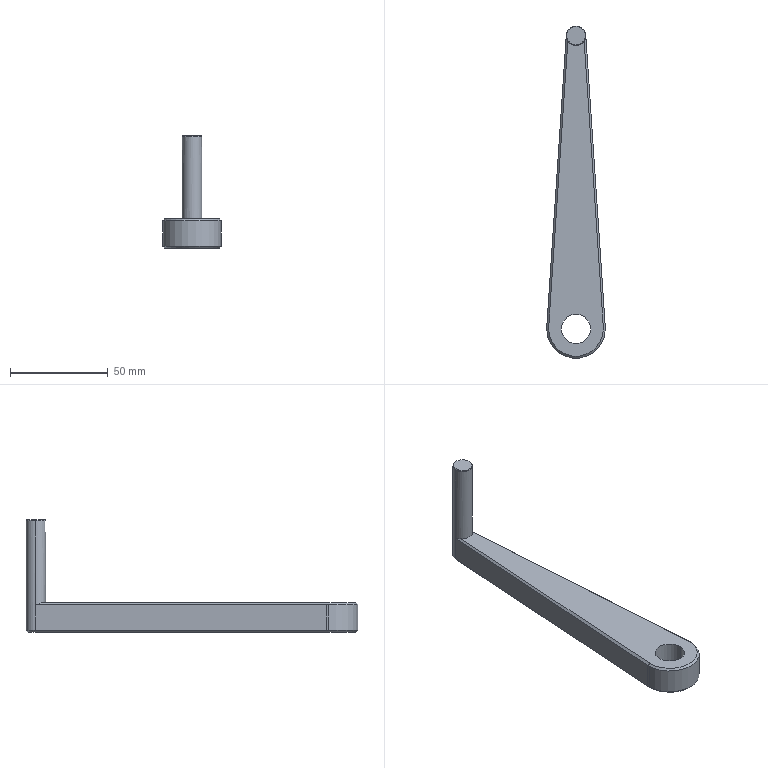Part | SolidWorks | features BaseBody 1 | 1 solid | 27 faces | box 30 x 170 x 57.5 mm | volume 51323 mm3 | cone 11 | plane 9 | cylinder 7 | commonest cylinder face diameters 30 x3 10 x2 15 x2
STEP:
#1=CARTESIAN_POINT('',(-4.823,150.,57.427));
#2=VERTEX_POINT('',#1);
#3=CARTESIAN_POINT('',(4.823,150.,57.427));
#4=VERTEX_POINT('',#3);
#5=CARTESIAN_POINT('',(0.,150.,57.427));
#6=DIRECTION('',(0.,0.,-1.));
#7=DIRECTION('',(-1.,0.,0.));
#8=AXIS2_PLACEMENT_3D('',#5,#6,#7);
#9=CIRCLE('',#8,4.823);
#10=EDGE_CURVE('',#2,#4,#9,.T.);
#11=ORIENTED_EDGE('',*,*,#10,.T.);
#12=CARTESIAN_POINT('',(5.,150.,57.));
#13=VERTEX_POINT('',#12);
#14=CARTESIAN_POINT('',(4.912,150.,57.213));
#15=DIRECTION('',(0.3827,0.,-0.9239));
#16=VECTOR('',#15,1000.);
#17=LINE('',#14,#16);
#18=EDGE_CURVE('',#4,#13,#17,.T.);
#19=ORIENTED_EDGE('',*,*,#18,.T.);
#20=CARTESIAN_POINT('',(-5.,150.,57.));
#21=VERTEX_POINT('',#20);
#22=CARTESIAN_POINT('',(0.,150.,57.));
#23=DIRECTION('',(0.,0.,1.));
#24=DIRECTION('',(-1.,0.,0.));
#25=AXIS2_PLACEMENT_3D('',#22,#23,#24);
#26=CIRCLE('',#25,5.);
#27=EDGE_CURVE('',#13,#21,#26,.T.);
#28=ORIENTED_EDGE('',*,*,#27,.T.);
#29=CARTESIAN_POINT('',(-4.912,150.,57.213));
#30=DIRECTION('',(-0.3827,0.,-0.9239));
#31=VECTOR('',#30,1000.);
#32=LINE('',#29,#31);
#33=EDGE_CURVE('',#2,#21,#32,.T.);
#34=ORIENTED_EDGE('',*,*,#33,.F.);
#35=EDGE_LOOP('',(#11,#19,#28,#34));
#36=FACE_OUTER_BOUND('',#35,.T.);
#37=CARTESIAN_POINT('',(0.,150.,57.213));
#38=DIRECTION('',(0.,0.,-1.));
#39=DIRECTION('',(-1.,0.,0.));
#40=AXIS2_PLACEMENT_3D('',#37,#38,#39);
#41=CONICAL_SURFACE('',#40,4.912,0.3927);
#42=ADVANCED_FACE('',(#36),#41,.T.);
#43=CARTESIAN_POINT('',(-4.75,150.,57.5));
#44=VERTEX_POINT('',#43);
#45=CARTESIAN_POINT('',(4.75,150.,57.5));
#46=VERTEX_POINT('',#45);
#47=CARTESIAN_POINT('',(0.,150.,57.5));
#48=DIRECTION('',(0.,0.,-1.));
#49=DIRECTION('',(-1.,0.,0.));
#50=AXIS2_PLACEMENT_3D('',#47,#48,#49);
#51=CIRCLE('',#50,4.75);
#52=EDGE_CURVE('',#44,#46,#51,.T.);
#53=ORIENTED_EDGE('',*,*,#52,.T.);
#54=CARTESIAN_POINT('',(4.875,150.,57.375));
#55=DIRECTION('',(0.7071,0.,-0.7071));
#56=VECTOR('',#55,1000.);
#57=LINE('',#54,#56);
#58=EDGE_CURVE('',#46,#4,#57,.T.);
#59=ORIENTED_EDGE('',*,*,#58,.T.);
#60=ORIENTED_EDGE('',*,*,#10,.F.);
#61=CARTESIAN_POINT('',(-4.875,150.,57.375));
#62=DIRECTION('',(-0.7071,0.,-0.7071));
#63=VECTOR('',#62,1000.);
#64=LINE('',#61,#63);
#65=EDGE_CURVE('',#44,#2,#64,.T.);
#66=ORIENTED_EDGE('',*,*,#65,.F.);
#67=EDGE_LOOP('',(#53,#59,#60,#66));
#68=FACE_OUTER_BOUND('',#67,.T.);
#69=CARTESIAN_POINT('',(0.,150.,57.375));
#70=DIRECTION('',(0.,0.,-1.));
#71=DIRECTION('',(-1.,0.,0.));
#72=AXIS2_PLACEMENT_3D('',#69,#70,#71);
#73=CONICAL_SURFACE('',#72,4.875,0.7854);
#74=ADVANCED_FACE('',(#68),#73,.T.);
#75=CARTESIAN_POINT('',(0.,150.,57.));
#76=DIRECTION('',(0.,0.,1.));
#77=DIRECTION('',(-1.,0.,0.));
#78=AXIS2_PLACEMENT_3D('',#75,#76,#77);
#79=CIRCLE('',#78,5.);
#80=EDGE_CURVE('',#21,#13,#79,.T.);
#81=ORIENTED_EDGE('',*,*,#80,.F.);
#82=CARTESIAN_POINT('',(-5.,150.,14.011));
#83=VERTEX_POINT('',#82);
#84=CARTESIAN_POINT('',(-5.,150.,0.));
#85=DIRECTION('',(0.,0.,-1.));
#86=VECTOR('',#85,1000.);
#87=LINE('',#84,#86);
#88=EDGE_CURVE('',#21,#83,#87,.T.);
#89=ORIENTED_EDGE('',*,*,#88,.T.);
#90=CARTESIAN_POINT('',(-4.191,147.273,15.));
#91=VERTEX_POINT('',#90);
#92=CARTESIAN_POINT('',(-4.191,147.273,15.));
#93=CARTESIAN_POINT('',(-4.723,148.091,14.415));
#94=CARTESIAN_POINT('',(-5.,149.025,14.076));
#95=CARTESIAN_POINT('',(-5.,150.,14.011));
#96=(BOUNDED_CURVE()B_SPLINE_CURVE(3,(#92,#93,#94,#95),.UNSPECIFIED.,.F.,.T.)B_SPLINE_CURVE_WITH_KNOTS((4,4),(2.498,3.075),.UNSPECIFIED.)CURVE()GEOMETRIC_REPRESENTATION_ITEM()RATIONAL_B_SPLINE_CURVE((1.,0.9725,0.9725,1.))REPRESENTATION_ITEM(''));
#97=EDGE_CURVE('',#91,#83,#96,.T.);
#98=ORIENTED_EDGE('',*,*,#97,.F.);
#99=CARTESIAN_POINT('',(4.191,147.273,15.));
#100=VERTEX_POINT('',#99);
#101=CARTESIAN_POINT('',(0.,150.,15.));
#102=DIRECTION('',(0.,0.,-1.));
#103=DIRECTION('',(-1.,0.,0.));
#104=AXIS2_PLACEMENT_3D('',#101,#102,#103);
#105=CIRCLE('',#104,5.);
#106=EDGE_CURVE('',#100,#91,#105,.T.);
#107=ORIENTED_EDGE('',*,*,#106,.F.);
#108=CARTESIAN_POINT('',(5.,150.,14.011));
#109=VERTEX_POINT('',#108);
#110=CARTESIAN_POINT('',(5.,150.,14.011));
#111=CARTESIAN_POINT('',(5.,149.025,14.076));
#112=CARTESIAN_POINT('',(4.723,148.091,14.415));
#113=CARTESIAN_POINT('',(4.191,147.273,15.));
#114=(BOUNDED_CURVE()B_SPLINE_CURVE(3,(#110,#111,#112,#113),.UNSPECIFIED.,.F.,.F.)B_SPLINE_CURVE_WITH_KNOTS((4,4),(0.06672,0.6435),.UNSPECIFIED.)CURVE()GEOMETRIC_REPRESENTATION_ITEM()RATIONAL_B_SPLINE_CURVE((1.,0.9725,0.9725,1.))REPRESENTATION_ITEM(''));
#115=EDGE_CURVE('',#109,#100,#114,.T.);
#116=ORIENTED_EDGE('',*,*,#115,.F.);
#117=CARTESIAN_POINT('',(5.,150.,0.));
#118=DIRECTION('',(0.,0.,-1.));
#119=VECTOR('',#118,1000.);
#120=LINE('',#117,#119);
#121=EDGE_CURVE('',#13,#109,#120,.T.);
#122=ORIENTED_EDGE('',*,*,#121,.F.);
#123=EDGE_LOOP('',(#81,#89,#98,#107,#116,#122));
#124=FACE_OUTER_BOUND('',#123,.T.);
#125=CARTESIAN_POINT('',(0.,150.,0.));
#126=DIRECTION('',(0.,0.,-1.));
#127=DIRECTION('',(1.,0.,0.));
#128=AXIS2_PLACEMENT_3D('',#125,#126,#127);
#129=CYLINDRICAL_SURFACE('',#128,5.);
#130=ADVANCED_FACE('',(#124),#129,.T.);
#131=CARTESIAN_POINT('',(-13.969,0.9333,0.));
#132=VERTEX_POINT('',#131);
#133=CARTESIAN_POINT('',(-14.,0.,0.));
#134=VERTEX_POINT('',#133);
#135=CARTESIAN_POINT('',(0.,0.,0.));
#136=DIRECTION('',(0.,0.,1.));
#137=DIRECTION('',(1.,0.,0.));
#138=AXIS2_PLACEMENT_3D('',#135,#136,#137);
#139=CIRCLE('',#138,14.);
#140=EDGE_CURVE('',#132,#134,#139,.T.);
#141=ORIENTED_EDGE('',*,*,#140,.T.);
#142=CARTESIAN_POINT('',(-15.,0.,1.));
#143=VERTEX_POINT('',#142);
#144=CARTESIAN_POINT('',(-14.5,0.,0.5));
#145=DIRECTION('',(-0.7071,0.,0.7071));
#146=VECTOR('',#145,1000.);
#147=LINE('',#144,#146);
#148=EDGE_CURVE('',#134,#143,#147,.T.);
#149=ORIENTED_EDGE('',*,*,#148,.T.);
#150=CARTESIAN_POINT('',(-14.967,1.,1.));
#151=VERTEX_POINT('',#150);
#152=CARTESIAN_POINT('',(0.,0.,1.));
#153=DIRECTION('',(0.,0.,-1.));
#154=DIRECTION('',(1.,0.,0.));
#155=AXIS2_PLACEMENT_3D('',#152,#153,#154);
#156=CIRCLE('',#155,15.);
#157=EDGE_CURVE('',#143,#151,#156,.T.);
#158=ORIENTED_EDGE('',*,*,#157,.T.);
#159=CARTESIAN_POINT('',(-13.969,0.9333,0.));
#160=DIRECTION('',(-0.7055,0.04714,0.7071));
#161=VECTOR('',#160,1000.);
#162=LINE('',#159,#161);
#163=EDGE_CURVE('',#132,#151,#162,.T.);
#164=ORIENTED_EDGE('',*,*,#163,.F.);
#165=EDGE_LOOP('',(#141,#149,#158,#164));
#166=FACE_OUTER_BOUND('',#165,.T.);
#167=CARTESIAN_POINT('',(0.,0.,0.5));
#168=DIRECTION('',(0.,0.,1.));
#169=DIRECTION('',(1.,0.,0.));
#170=AXIS2_PLACEMENT_3D('',#167,#168,#169);
#171=CONICAL_SURFACE('',#170,14.5,0.7854);
#172=ADVANCED_FACE('',(#166),#171,.T.);
#173=ORIENTED_EDGE('',*,*,#148,.F.);
#174=CARTESIAN_POINT('',(14.,0.,0.));
#175=VERTEX_POINT('',#174);
#176=CARTESIAN_POINT('',(0.,0.,0.));
#177=DIRECTION('',(0.,0.,1.));
#178=DIRECTION('',(1.,0.,0.));
#179=AXIS2_PLACEMENT_3D('',#176,#177,#178);
#180=CIRCLE('',#179,14.);
#181=EDGE_CURVE('',#134,#175,#180,.T.);
#182=ORIENTED_EDGE('',*,*,#181,.T.);
#183=CARTESIAN_POINT('',(15.,0.,1.));
#184=VERTEX_POINT('',#183);
#185=CARTESIAN_POINT('',(14.5,0.,0.5));
#186=DIRECTION('',(0.7071,0.,0.7071));
#187=VECTOR('',#186,1000.);
#188=LINE('',#185,#187);
#189=EDGE_CURVE('',#175,#184,#188,.T.);
#190=ORIENTED_EDGE('',*,*,#189,.T.);
#191=CARTESIAN_POINT('',(0.,0.,1.));
#192=DIRECTION('',(0.,0.,-1.));
#193=DIRECTION('',(1.,0.,0.));
#194=AXIS2_PLACEMENT_3D('',#191,#192,#193);
#195=CIRCLE('',#194,15.);
#196=EDGE_CURVE('',#184,#143,#195,.T.);
#197=ORIENTED_EDGE('',*,*,#196,.T.);
#198=EDGE_LOOP('',(#173,#182,#190,#197));
#199=FACE_OUTER_BOUND('',#198,.T.);
#200=CARTESIAN_POINT('',(0.,0.,0.5));
#201=DIRECTION('',(0.,0.,1.));
#202=DIRECTION('',(1.,0.,0.));
#203=AXIS2_PLACEMENT_3D('',#200,#201,#202);
#204=CONICAL_SURFACE('',#203,14.5,0.7854);
#205=ADVANCED_FACE('',(#199),#204,.T.);
#206=CARTESIAN_POINT('',(-15.,0.,14.));
#207=VERTEX_POINT('',#206);
#208=CARTESIAN_POINT('',(15.,0.,14.));
#209=VERTEX_POINT('',#208);
#210=CARTESIAN_POINT('',(0.,0.,14.));
#211=DIRECTION('',(0.,0.,1.));
#212=DIRECTION('',(1.,0.,0.));
#213=AXIS2_PLACEMENT_3D('',#210,#211,#212);
#214=CIRCLE('',#213,15.);
#215=EDGE_CURVE('',#207,#209,#214,.T.);
#216=ORIENTED_EDGE('',*,*,#215,.F.);
#217=CARTESIAN_POINT('',(-15.,0.,0.));
#218=DIRECTION('',(0.,0.,-1.));
#219=VECTOR('',#218,1000.);
#220=LINE('',#217,#219);
#221=EDGE_CURVE('',#207,#143,#220,.T.);
#222=ORIENTED_EDGE('',*,*,#221,.T.);
#223=ORIENTED_EDGE('',*,*,#196,.F.);
#224=CARTESIAN_POINT('',(15.,0.,0.));
#225=DIRECTION('',(0.,0.,-1.));
#226=VECTOR('',#225,1000.);
#227=LINE('',#224,#226);
#228=EDGE_CURVE('',#209,#184,#227,.T.);
#229=ORIENTED_EDGE('',*,*,#228,.F.);
#230=EDGE_LOOP('',(#216,#222,#223,#229));
#231=FACE_OUTER_BOUND('',#230,.T.);
#232=CARTESIAN_POINT('',(0.,0.,0.));
#233=DIRECTION('',(0.,0.,-1.));
#234=DIRECTION('',(1.,0.,0.));
#235=AXIS2_PLACEMENT_3D('',#232,#233,#234);
#236=CYLINDRICAL_SURFACE('',#235,15.);
#237=ADVANCED_FACE('',(#231),#236,.T.);
#238=CARTESIAN_POINT('',(14.967,1.,14.));
#239=VERTEX_POINT('',#238);
#240=CARTESIAN_POINT('',(0.,0.,14.));
#241=DIRECTION('',(0.,0.,1.));
#242=DIRECTION('',(1.,0.,0.));
#243=AXIS2_PLACEMENT_3D('',#240,#241,#242);
#244=CIRCLE('',#243,15.);
#245=EDGE_CURVE('',#209,#239,#244,.T.);
#246=ORIENTED_EDGE('',*,*,#245,.F.);
#247=ORIENTED_EDGE('',*,*,#228,.T.);
#248=CARTESIAN_POINT('',(14.967,1.,1.));
#249=VERTEX_POINT('',#248);
#250=CARTESIAN_POINT('',(0.,0.,1.));
#251=DIRECTION('',(0.,0.,-1.));
#252=DIRECTION('',(1.,0.,0.));
#253=AXIS2_PLACEMENT_3D('',#250,#251,#252);
#254=CIRCLE('',#253,15.);
#255=EDGE_CURVE('',#249,#184,#254,.T.);
#256=ORIENTED_EDGE('',*,*,#255,.F.);
#257=CARTESIAN_POINT('',(14.967,1.,0.));
#258=DIRECTION('',(0.,0.,1.));
#259=VECTOR('',#258,1000.);
#260=LINE('',#257,#259);
#261=EDGE_CURVE('',#249,#239,#260,.T.);
#262=ORIENTED_EDGE('',*,*,#261,.T.);
#263=EDGE_LOOP('',(#246,#247,#256,#262));
#264=FACE_OUTER_BOUND('',#263,.T.);
#265=CARTESIAN_POINT('',(0.,0.,0.));
#266=DIRECTION('',(0.,0.,-1.));
#267=DIRECTION('',(1.,0.,0.));
#268=AXIS2_PLACEMENT_3D('',#265,#266,#267);
#269=CYLINDRICAL_SURFACE('',#268,15.);
#270=ADVANCED_FACE('',(#264),#269,.T.);
#271=CARTESIAN_POINT('',(14.,0.,15.));
#272=VERTEX_POINT('',#271);
#273=CARTESIAN_POINT('',(-14.,0.,15.));
#274=VERTEX_POINT('',#273);
#275=CARTESIAN_POINT('',(0.,0.,15.));
#276=DIRECTION('',(0.,0.,-1.));
#277=DIRECTION('',(1.,0.,0.));
#278=AXIS2_PLACEMENT_3D('',#275,#276,#277);
#279=CIRCLE('',#278,14.);
#280=EDGE_CURVE('',#272,#274,#279,.T.);
#281=ORIENTED_EDGE('',*,*,#280,.T.);
#282=CARTESIAN_POINT('',(-14.5,0.,14.5));
#283=DIRECTION('',(-0.7071,0.,-0.7071));
#284=VECTOR('',#283,1000.);
#285=LINE('',#282,#284);
#286=EDGE_CURVE('',#274,#207,#285,.T.);
#287=ORIENTED_EDGE('',*,*,#286,.T.);
#288=ORIENTED_EDGE('',*,*,#215,.T.);
#289=CARTESIAN_POINT('',(14.5,0.,14.5));
#290=DIRECTION('',(0.7071,0.,-0.7071));
#291=VECTOR('',#290,1000.);
#292=LINE('',#289,#291);
#293=EDGE_CURVE('',#272,#209,#292,.T.);
#294=ORIENTED_EDGE('',*,*,#293,.F.);
#295=EDGE_LOOP('',(#281,#287,#288,#294));
#296=FACE_OUTER_BOUND('',#295,.T.);
#297=CARTESIAN_POINT('',(0.,0.,14.5));
#298=DIRECTION('',(0.,0.,-1.));
#299=DIRECTION('',(1.,0.,0.));
#300=AXIS2_PLACEMENT_3D('',#297,#298,#299);
#301=CONICAL_SURFACE('',#300,14.5,0.7854);
#302=ADVANCED_FACE('',(#296),#301,.T.);
#303=CARTESIAN_POINT('',(13.969,0.9333,15.));
#304=VERTEX_POINT('',#303);
#305=CARTESIAN_POINT('',(0.,0.,15.));
#306=DIRECTION('',(0.,0.,-1.));
#307=DIRECTION('',(1.,0.,0.));
#308=AXIS2_PLACEMENT_3D('',#305,#306,#307);
#309=CIRCLE('',#308,14.);
#310=EDGE_CURVE('',#304,#272,#309,.T.);
#311=ORIENTED_EDGE('',*,*,#310,.T.);
#312=ORIENTED_EDGE('',*,*,#293,.T.);
#313=ORIENTED_EDGE('',*,*,#245,.T.);
#314=CARTESIAN_POINT('',(14.967,1.,14.));
#315=DIRECTION('',(-0.7055,-0.04714,0.7071));
#316=VECTOR('',#315,1000.);
#317=LINE('',#314,#316);
#318=EDGE_CURVE('',#239,#304,#317,.T.);
#319=ORIENTED_EDGE('',*,*,#318,.T.);
#320=EDGE_LOOP('',(#311,#312,#313,#319));
#321=FACE_OUTER_BOUND('',#320,.T.);
#322=CARTESIAN_POINT('',(0.,0.,14.5));
#323=DIRECTION('',(0.,0.,-1.));
#324=DIRECTION('',(1.,0.,0.));
#325=AXIS2_PLACEMENT_3D('',#322,#323,#324);
#326=CONICAL_SURFACE('',#325,14.5,0.7854);
#327=ADVANCED_FACE('',(#321),#326,.T.);
#328=CARTESIAN_POINT('',(7.5,0.,0.));
#329=VERTEX_POINT('',#328);
#330=CARTESIAN_POINT('',(-7.5,0.,0.));
#331=VERTEX_POINT('',#330);
#332=CARTESIAN_POINT('',(0.,0.,0.));
#333=DIRECTION('',(0.,0.,1.));
#334=DIRECTION('',(-1.,0.,0.));
#335=AXIS2_PLACEMENT_3D('',#332,#333,#334);
#336=CIRCLE('',#335,7.5);
#337=EDGE_CURVE('',#329,#331,#336,.T.);
#338=ORIENTED_EDGE('',*,*,#337,.F.);
#339=CARTESIAN_POINT('',(7.5,0.,15.));
#340=VERTEX_POINT('',#339);
#341=CARTESIAN_POINT('',(7.5,0.,15.));
#342=DIRECTION('',(0.,0.,1.));
#343=VECTOR('',#342,1000.);
#344=LINE('',#341,#343);
#345=EDGE_CURVE('',#329,#340,#344,.T.);
#346=ORIENTED_EDGE('',*,*,#345,.T.);
#347=CARTESIAN_POINT('',(-7.5,0.,15.));
#348=VERTEX_POINT('',#347);
#349=CARTESIAN_POINT('',(0.,0.,15.));
#350=DIRECTION('',(0.,0.,-1.));
#351=DIRECTION('',(-1.,0.,0.));
#352=AXIS2_PLACEMENT_3D('',#349,#350,#351);
#353=CIRCLE('',#352,7.5);
#354=EDGE_CURVE('',#348,#340,#353,.T.);
#355=ORIENTED_EDGE('',*,*,#354,.F.);
#356=CARTESIAN_POINT('',(-7.5,0.,15.));
#357=DIRECTION('',(0.,0.,1.));
#358=VECTOR('',#357,1000.);
#359=LINE('',#356,#358);
#360=EDGE_CURVE('',#331,#348,#359,.T.);
#361=ORIENTED_EDGE('',*,*,#360,.F.);
#362=EDGE_LOOP('',(#338,#346,#355,#361));
#363=FACE_OUTER_BOUND('',#362,.T.);
#364=CARTESIAN_POINT('',(0.,0.,15.));
#365=DIRECTION('',(0.,0.,1.));
#366=DIRECTION('',(-1.,0.,0.));
#367=AXIS2_PLACEMENT_3D('',#364,#365,#366);
#368=CYLINDRICAL_SURFACE('',#367,7.5);
#369=ADVANCED_FACE('',(#363),#368,.F.);
#370=CARTESIAN_POINT('',(3.991,150.267,0.));
#371=VERTEX_POINT('',#370);
#372=CARTESIAN_POINT('',(4.989,150.333,1.));
#373=VERTEX_POINT('',#372);
#374=CARTESIAN_POINT('',(3.991,150.267,0.));
#375=DIRECTION('',(0.7055,0.04714,0.7071));
#376=VECTOR('',#375,1000.);
#377=LINE('',#374,#376);
#378=EDGE_CURVE('',#371,#373,#377,.T.);
#379=ORIENTED_EDGE('',*,*,#378,.T.);
#380=CARTESIAN_POINT('',(9.978,75.667,1.));
#381=DIRECTION('',(0.06667,-0.9978,0.));
#382=VECTOR('',#381,1000.);
#383=LINE('',#380,#382);
#384=EDGE_CURVE('',#373,#249,#383,.T.);
#385=ORIENTED_EDGE('',*,*,#384,.T.);
#386=CARTESIAN_POINT('',(13.969,0.9333,0.));
#387=VERTEX_POINT('',#386);
#388=CARTESIAN_POINT('',(14.967,1.,1.));
#389=DIRECTION('',(-0.7055,-0.04714,-0.7071));
#390=VECTOR('',#389,1000.);
#391=LINE('',#388,#390);
#392=EDGE_CURVE('',#249,#387,#391,.T.);
#393=ORIENTED_EDGE('',*,*,#392,.T.);
#394=CARTESIAN_POINT('',(8.98,75.6,0.));
#395=DIRECTION('',(-0.06667,0.9978,0.));
#396=VECTOR('',#395,1000.);
#397=LINE('',#394,#396);
#398=EDGE_CURVE('',#387,#371,#397,.T.);
#399=ORIENTED_EDGE('',*,*,#398,.T.);
#400=EDGE_LOOP('',(#379,#385,#393,#399));
#401=FACE_OUTER_BOUND('',#400,.T.);
#402=CARTESIAN_POINT('',(9.479,75.633,0.5));
#403=DIRECTION('',(0.7055,0.04714,-0.7071));
#404=DIRECTION('',(0.,-0.9978,-0.06652));
#405=AXIS2_PLACEMENT_3D('',#402,#403,#404);
#406=PLANE('',#405);
#407=ADVANCED_FACE('',(#401),#406,.T.);
#408=CARTESIAN_POINT('',(-3.991,150.267,0.));
#409=VERTEX_POINT('',#408);
#410=CARTESIAN_POINT('',(-4.989,150.333,1.));
#411=VERTEX_POINT('',#410);
#412=CARTESIAN_POINT('',(-3.991,150.267,0.));
#413=DIRECTION('',(-0.7055,0.04714,0.7071));
#414=VECTOR('',#413,1000.);
#415=LINE('',#412,#414);
#416=EDGE_CURVE('',#409,#411,#415,.T.);
#417=ORIENTED_EDGE('',*,*,#416,.T.);
#418=CARTESIAN_POINT('',(0.,150.,1.));
#419=DIRECTION('',(0.,0.,-1.));
#420=DIRECTION('',(1.,0.,0.));
#421=AXIS2_PLACEMENT_3D('',#418,#419,#420);
#422=CIRCLE('',#421,5.);
#423=EDGE_CURVE('',#411,#373,#422,.T.);
#424=ORIENTED_EDGE('',*,*,#423,.T.);
#425=ORIENTED_EDGE('',*,*,#378,.F.);
#426=CARTESIAN_POINT('',(0.,150.,0.));
#427=DIRECTION('',(0.,0.,1.));
#428=DIRECTION('',(1.,0.,0.));
#429=AXIS2_PLACEMENT_3D('',#426,#427,#428);
#430=CIRCLE('',#429,4.);
#431=EDGE_CURVE('',#371,#409,#430,.T.);
#432=ORIENTED_EDGE('',*,*,#431,.T.);
#433=EDGE_LOOP('',(#417,#424,#425,#432));
#434=FACE_OUTER_BOUND('',#433,.T.);
#435=CARTESIAN_POINT('',(0.,150.,0.5));
#436=DIRECTION('',(0.,0.,1.));
#437=DIRECTION('',(1.,0.,0.));
#438=AXIS2_PLACEMENT_3D('',#435,#436,#437);
#439=CONICAL_SURFACE('',#438,4.5,0.7854);
#440=ADVANCED_FACE('',(#434),#439,.T.);
#441=ORIENTED_EDGE('',*,*,#163,.T.);
#442=CARTESIAN_POINT('',(-4.989,150.333,1.));
#443=DIRECTION('',(0.06667,0.9978,0.));
#444=VECTOR('',#443,1000.);
#445=LINE('',#442,#444);
#446=EDGE_CURVE('',#151,#411,#445,.T.);
#447=ORIENTED_EDGE('',*,*,#446,.T.);
#448=ORIENTED_EDGE('',*,*,#416,.F.);
#449=CARTESIAN_POINT('',(-3.991,150.267,0.));
#450=DIRECTION('',(-0.06667,-0.9978,0.));
#451=VECTOR('',#450,1000.);
#452=LINE('',#449,#451);
#453=EDGE_CURVE('',#409,#132,#452,.T.);
#454=ORIENTED_EDGE('',*,*,#453,.T.);
#455=EDGE_LOOP('',(#441,#447,#448,#454));
#456=FACE_OUTER_BOUND('',#455,.T.);
#457=CARTESIAN_POINT('',(-4.49,150.3,0.5));
#458=DIRECTION('',(-0.7055,0.04714,-0.7071));
#459=DIRECTION('',(-0.7079,0.,0.7063));
#460=AXIS2_PLACEMENT_3D('',#457,#458,#459);
#461=PLANE('',#460);
#462=ADVANCED_FACE('',(#456),#461,.T.);
#463=ORIENTED_EDGE('',*,*,#384,.F.);
#464=CARTESIAN_POINT('',(4.989,150.333,14.));
#465=VERTEX_POINT('',#464);
#466=CARTESIAN_POINT('',(4.989,150.333,0.));
#467=DIRECTION('',(0.,0.,1.));
#468=VECTOR('',#467,1000.);
#469=LINE('',#466,#468);
#470=EDGE_CURVE('',#373,#465,#469,.T.);
#471=ORIENTED_EDGE('',*,*,#470,.T.);
#472=CARTESIAN_POINT('',(9.978,75.667,14.));
#473=DIRECTION('',(-0.06667,0.9978,0.));
#474=VECTOR('',#473,1000.);
#475=LINE('',#472,#474);
#476=EDGE_CURVE('',#239,#465,#475,.T.);
#477=ORIENTED_EDGE('',*,*,#476,.F.);
#478=ORIENTED_EDGE('',*,*,#261,.F.);
#479=EDGE_LOOP('',(#463,#471,#477,#478));
#480=FACE_OUTER_BOUND('',#479,.T.);
#481=CARTESIAN_POINT('',(14.967,1.,0.));
#482=DIRECTION('',(0.9978,0.06667,0.));
#483=DIRECTION('',(0.,0.,-1.));
#484=AXIS2_PLACEMENT_3D('',#481,#482,#483);
#485=PLANE('',#484);
#486=ADVANCED_FACE('',(#480),#485,.T.);
#487=CARTESIAN_POINT('',(0.,0.,0.));
#488=DIRECTION('',(0.,0.,1.));
#489=DIRECTION('',(-1.,0.,0.));
#490=AXIS2_PLACEMENT_3D('',#487,#488,#489);
#491=CIRCLE('',#490,7.5);
#492=EDGE_CURVE('',#331,#329,#491,.T.);
#493=ORIENTED_EDGE('',*,*,#492,.T.);
#494=ORIENTED_EDGE('',*,*,#337,.T.);
#495=EDGE_LOOP('',(#493,#494));
#496=FACE_BOUND('',#495,.T.);
#497=ORIENTED_EDGE('',*,*,#398,.F.);
#498=CARTESIAN_POINT('',(0.,0.,0.));
#499=DIRECTION('',(0.,0.,1.));
#500=DIRECTION('',(1.,0.,0.));
#501=AXIS2_PLACEMENT_3D('',#498,#499,#500);
#502=CIRCLE('',#501,14.);
#503=EDGE_CURVE('',#175,#387,#502,.T.);
#504=ORIENTED_EDGE('',*,*,#503,.F.);
#505=ORIENTED_EDGE('',*,*,#181,.F.);
#506=ORIENTED_EDGE('',*,*,#140,.F.);
#507=ORIENTED_EDGE('',*,*,#453,.F.);
#508=ORIENTED_EDGE('',*,*,#431,.F.);
#509=EDGE_LOOP('',(#497,#504,#505,#506,#507,#508));
#510=FACE_OUTER_BOUND('',#509,.T.);
#511=CARTESIAN_POINT('',(0.,150.,0.));
#512=DIRECTION('',(0.,0.,1.));
#513=DIRECTION('',(1.,0.,0.));
#514=AXIS2_PLACEMENT_3D('',#511,#512,#513);
#515=PLANE('',#514);
#516=ADVANCED_FACE('',(#496,#510),#515,.F.);
#517=ORIENTED_EDGE('',*,*,#97,.T.);
#518=CARTESIAN_POINT('',(-4.989,150.333,14.));
#519=VERTEX_POINT('',#518);
#520=CARTESIAN_POINT('',(-5.,150.,14.011));
#521=CARTESIAN_POINT('',(-5.,150.111,14.004));
#522=CARTESIAN_POINT('',(-4.996,150.222,14.));
#523=CARTESIAN_POINT('',(-4.989,150.333,14.));
#524=(BOUNDED_CURVE()B_SPLINE_CURVE(3,(#520,#521,#522,#523),.UNSPECIFIED.,.F.,.F.)B_SPLINE_CURVE_WITH_KNOTS((4,4),(3.075,3.142),.UNSPECIFIED.)CURVE()GEOMETRIC_REPRESENTATION_ITEM()RATIONAL_B_SPLINE_CURVE((1.,0.9996,0.9996,1.))REPRESENTATION_ITEM(''));
#525=EDGE_CURVE('',#83,#519,#524,.T.);
#526=ORIENTED_EDGE('',*,*,#525,.T.);
#527=CARTESIAN_POINT('',(-14.967,1.,14.));
#528=VERTEX_POINT('',#527);
#529=CARTESIAN_POINT('',(-4.989,150.333,14.));
#530=DIRECTION('',(-0.06667,-0.9978,0.));
#531=VECTOR('',#530,1000.);
#532=LINE('',#529,#531);
#533=EDGE_CURVE('',#519,#528,#532,.T.);
#534=ORIENTED_EDGE('',*,*,#533,.T.);
#535=CARTESIAN_POINT('',(-13.969,0.9333,15.));
#536=VERTEX_POINT('',#535);
#537=CARTESIAN_POINT('',(-14.967,1.,14.));
#538=DIRECTION('',(0.7055,-0.04714,0.7071));
#539=VECTOR('',#538,1000.);
#540=LINE('',#537,#539);
#541=EDGE_CURVE('',#528,#536,#540,.T.);
#542=ORIENTED_EDGE('',*,*,#541,.T.);
#543=CARTESIAN_POINT('',(-3.991,150.267,15.));
#544=DIRECTION('',(0.06667,0.9978,0.));
#545=VECTOR('',#544,1000.);
#546=LINE('',#543,#545);
#547=EDGE_CURVE('',#536,#91,#546,.T.);
#548=ORIENTED_EDGE('',*,*,#547,.T.);
#549=EDGE_LOOP('',(#517,#526,#534,#542,#548));
#550=FACE_OUTER_BOUND('',#549,.T.);
#551=CARTESIAN_POINT('',(-4.49,150.3,14.5));
#552=DIRECTION('',(-0.7055,0.04714,0.7071));
#553=DIRECTION('',(0.06667,0.9978,0.));
#554=AXIS2_PLACEMENT_3D('',#551,#552,#553);
#555=PLANE('',#554);
#556=ADVANCED_FACE('',(#550),#555,.T.);
#557=CARTESIAN_POINT('',(4.989,150.333,14.));
#558=CARTESIAN_POINT('',(4.996,150.222,14.));
#559=CARTESIAN_POINT('',(5.,150.111,14.004));
#560=CARTESIAN_POINT('',(5.,150.,14.011));
#561=(BOUNDED_CURVE()B_SPLINE_CURVE(3,(#557,#558,#559,#560),.UNSPECIFIED.,.F.,.T.)B_SPLINE_CURVE_WITH_KNOTS((4,4),(0.,0.06672),.UNSPECIFIED.)CURVE()GEOMETRIC_REPRESENTATION_ITEM()RATIONAL_B_SPLINE_CURVE((1.,0.9996,0.9996,1.))REPRESENTATION_ITEM(''));
#562=EDGE_CURVE('',#465,#109,#561,.T.);
#563=ORIENTED_EDGE('',*,*,#562,.T.);
#564=ORIENTED_EDGE('',*,*,#115,.T.);
#565=CARTESIAN_POINT('',(8.98,75.6,15.));
#566=DIRECTION('',(0.06667,-0.9978,0.));
#567=VECTOR('',#566,1000.);
#568=LINE('',#565,#567);
#569=EDGE_CURVE('',#100,#304,#568,.T.);
#570=ORIENTED_EDGE('',*,*,#569,.T.);
#571=ORIENTED_EDGE('',*,*,#318,.F.);
#572=ORIENTED_EDGE('',*,*,#476,.T.);
#573=EDGE_LOOP('',(#563,#564,#570,#571,#572));
#574=FACE_OUTER_BOUND('',#573,.T.);
#575=CARTESIAN_POINT('',(9.479,75.633,14.5));
#576=DIRECTION('',(0.7055,0.04714,0.7071));
#577=DIRECTION('',(0.06667,-0.9978,0.));
#578=AXIS2_PLACEMENT_3D('',#575,#576,#577);
#579=PLANE('',#578);
#580=ADVANCED_FACE('',(#574),#579,.T.);
#581=ORIENTED_EDGE('',*,*,#446,.F.);
#582=CARTESIAN_POINT('',(-14.967,1.,0.));
#583=DIRECTION('',(0.,0.,1.));
#584=VECTOR('',#583,1000.);
#585=LINE('',#582,#584);
#586=EDGE_CURVE('',#151,#528,#585,.T.);
#587=ORIENTED_EDGE('',*,*,#586,.T.);
#588=ORIENTED_EDGE('',*,*,#533,.F.);
#589=CARTESIAN_POINT('',(-4.989,150.333,0.));
#590=DIRECTION('',(0.,0.,1.));
#591=VECTOR('',#590,1000.);
#592=LINE('',#589,#591);
#593=EDGE_CURVE('',#411,#519,#592,.T.);
#594=ORIENTED_EDGE('',*,*,#593,.F.);
#595=EDGE_LOOP('',(#581,#587,#588,#594));
#596=FACE_OUTER_BOUND('',#595,.T.);
#597=CARTESIAN_POINT('',(-4.989,150.333,0.));
#598=DIRECTION('',(-0.9978,0.06667,0.));
#599=DIRECTION('',(0.,0.,1.));
#600=AXIS2_PLACEMENT_3D('',#597,#598,#599);
#601=PLANE('',#600);
#602=ADVANCED_FACE('',(#596),#601,.T.);
#603=ORIENTED_EDGE('',*,*,#52,.F.);
#604=CARTESIAN_POINT('',(0.,150.,57.5));
#605=DIRECTION('',(0.,0.,-1.));
#606=DIRECTION('',(-1.,0.,0.));
#607=AXIS2_PLACEMENT_3D('',#604,#605,#606);
#608=CIRCLE('',#607,4.75);
#609=EDGE_CURVE('',#46,#44,#608,.T.);
#610=ORIENTED_EDGE('',*,*,#609,.F.);
#611=EDGE_LOOP('',(#603,#610));
#612=FACE_OUTER_BOUND('',#611,.T.);
#613=CARTESIAN_POINT('',(0.,150.,57.5));
#614=DIRECTION('',(0.,0.,1.));
#615=DIRECTION('',(1.,0.,0.));
#616=AXIS2_PLACEMENT_3D('',#613,#614,#615);
#617=PLANE('',#616);
#618=ADVANCED_FACE('',(#612),#617,.T.);
#619=ORIENTED_EDGE('',*,*,#354,.T.);
#620=CARTESIAN_POINT('',(0.,0.,15.));
#621=DIRECTION('',(0.,0.,-1.));
#622=DIRECTION('',(-1.,0.,0.));
#623=AXIS2_PLACEMENT_3D('',#620,#621,#622);
#624=CIRCLE('',#623,7.5);
#625=EDGE_CURVE('',#340,#348,#624,.T.);
#626=ORIENTED_EDGE('',*,*,#625,.T.);
#627=EDGE_LOOP('',(#619,#626));
#628=FACE_BOUND('',#627,.T.);
#629=ORIENTED_EDGE('',*,*,#569,.F.);
#630=ORIENTED_EDGE('',*,*,#106,.T.);
#631=ORIENTED_EDGE('',*,*,#547,.F.);
#632=CARTESIAN_POINT('',(0.,0.,15.));
#633=DIRECTION('',(0.,0.,-1.));
#634=DIRECTION('',(1.,0.,0.));
#635=AXIS2_PLACEMENT_3D('',#632,#633,#634);
#636=CIRCLE('',#635,14.);
#637=EDGE_CURVE('',#274,#536,#636,.T.);
#638=ORIENTED_EDGE('',*,*,#637,.F.);
#639=ORIENTED_EDGE('',*,*,#280,.F.);
#640=ORIENTED_EDGE('',*,*,#310,.F.);
#641=EDGE_LOOP('',(#629,#630,#631,#638,#639,#640));
#642=FACE_OUTER_BOUND('',#641,.T.);
#643=CARTESIAN_POINT('',(0.,150.,15.));
#644=DIRECTION('',(0.,0.,1.));
#645=DIRECTION('',(1.,0.,0.));
#646=AXIS2_PLACEMENT_3D('',#643,#644,#645);
#647=PLANE('',#646);
#648=ADVANCED_FACE('',(#628,#642),#647,.T.);
#649=ORIENTED_EDGE('',*,*,#345,.F.);
#650=ORIENTED_EDGE('',*,*,#492,.F.);
#651=ORIENTED_EDGE('',*,*,#360,.T.);
#652=ORIENTED_EDGE('',*,*,#625,.F.);
#653=EDGE_LOOP('',(#649,#650,#651,#652));
#654=FACE_OUTER_BOUND('',#653,.T.);
#655=CARTESIAN_POINT('',(0.,0.,15.));
#656=DIRECTION('',(0.,0.,1.));
#657=DIRECTION('',(-1.,0.,0.));
#658=AXIS2_PLACEMENT_3D('',#655,#656,#657);
#659=CYLINDRICAL_SURFACE('',#658,7.5);
#660=ADVANCED_FACE('',(#654),#659,.F.);
#661=ORIENTED_EDGE('',*,*,#286,.F.);
#662=ORIENTED_EDGE('',*,*,#637,.T.);
#663=ORIENTED_EDGE('',*,*,#541,.F.);
#664=CARTESIAN_POINT('',(0.,0.,14.));
#665=DIRECTION('',(0.,0.,1.));
#666=DIRECTION('',(1.,0.,0.));
#667=AXIS2_PLACEMENT_3D('',#664,#665,#666);
#668=CIRCLE('',#667,15.);
#669=EDGE_CURVE('',#528,#207,#668,.T.);
#670=ORIENTED_EDGE('',*,*,#669,.T.);
#671=EDGE_LOOP('',(#661,#662,#663,#670));
#672=FACE_OUTER_BOUND('',#671,.T.);
#673=CARTESIAN_POINT('',(0.,0.,14.5));
#674=DIRECTION('',(0.,0.,-1.));
#675=DIRECTION('',(1.,0.,0.));
#676=AXIS2_PLACEMENT_3D('',#673,#674,#675);
#677=CONICAL_SURFACE('',#676,14.5,0.7854);
#678=ADVANCED_FACE('',(#672),#677,.T.);
#679=ORIENTED_EDGE('',*,*,#221,.F.);
#680=ORIENTED_EDGE('',*,*,#669,.F.);
#681=ORIENTED_EDGE('',*,*,#586,.F.);
#682=ORIENTED_EDGE('',*,*,#157,.F.);
#683=EDGE_LOOP('',(#679,#680,#681,#682));
#684=FACE_OUTER_BOUND('',#683,.T.);
#685=CARTESIAN_POINT('',(0.,0.,0.));
#686=DIRECTION('',(0.,0.,-1.));
#687=DIRECTION('',(1.,0.,0.));
#688=AXIS2_PLACEMENT_3D('',#685,#686,#687);
#689=CYLINDRICAL_SURFACE('',#688,15.);
#690=ADVANCED_FACE('',(#684),#689,.T.);
#691=ORIENTED_EDGE('',*,*,#189,.F.);
#692=ORIENTED_EDGE('',*,*,#503,.T.);
#693=ORIENTED_EDGE('',*,*,#392,.F.);
#694=ORIENTED_EDGE('',*,*,#255,.T.);
#695=EDGE_LOOP('',(#691,#692,#693,#694));
#696=FACE_OUTER_BOUND('',#695,.T.);
#697=CARTESIAN_POINT('',(0.,0.,0.5));
#698=DIRECTION('',(0.,0.,1.));
#699=DIRECTION('',(1.,0.,0.));
#700=AXIS2_PLACEMENT_3D('',#697,#698,#699);
#701=CONICAL_SURFACE('',#700,14.5,0.7854);
#702=ADVANCED_FACE('',(#696),#701,.T.);
#703=ORIENTED_EDGE('',*,*,#88,.F.);
#704=ORIENTED_EDGE('',*,*,#27,.F.);
#705=ORIENTED_EDGE('',*,*,#121,.T.);
#706=ORIENTED_EDGE('',*,*,#562,.F.);
#707=ORIENTED_EDGE('',*,*,#470,.F.);
#708=ORIENTED_EDGE('',*,*,#423,.F.);
#709=ORIENTED_EDGE('',*,*,#593,.T.);
#710=ORIENTED_EDGE('',*,*,#525,.F.);
#711=EDGE_LOOP('',(#703,#704,#705,#706,#707,#708,#709,#710));
#712=FACE_OUTER_BOUND('',#711,.T.);
#713=CARTESIAN_POINT('',(0.,150.,0.));
#714=DIRECTION('',(0.,0.,-1.));
#715=DIRECTION('',(1.,0.,0.));
#716=AXIS2_PLACEMENT_3D('',#713,#714,#715);
#717=CYLINDRICAL_SURFACE('',#716,5.);
#718=ADVANCED_FACE('',(#712),#717,.T.);
#719=ORIENTED_EDGE('',*,*,#58,.F.);
#720=ORIENTED_EDGE('',*,*,#609,.T.);
#721=ORIENTED_EDGE('',*,*,#65,.T.);
#722=CARTESIAN_POINT('',(0.,150.,57.427));
#723=DIRECTION('',(0.,0.,-1.));
#724=DIRECTION('',(-1.,0.,0.));
#725=AXIS2_PLACEMENT_3D('',#722,#723,#724);
#726=CIRCLE('',#725,4.823);
#727=EDGE_CURVE('',#4,#2,#726,.T.);
#728=ORIENTED_EDGE('',*,*,#727,.F.);
#729=EDGE_LOOP('',(#719,#720,#721,#728));
#730=FACE_OUTER_BOUND('',#729,.T.);
#731=CARTESIAN_POINT('',(0.,150.,57.375));
#732=DIRECTION('',(0.,0.,-1.));
#733=DIRECTION('',(-1.,0.,0.));
#734=AXIS2_PLACEMENT_3D('',#731,#732,#733);
#735=CONICAL_SURFACE('',#734,4.875,0.7854);
#736=ADVANCED_FACE('',(#730),#735,.T.);
#737=ORIENTED_EDGE('',*,*,#18,.F.);
#738=ORIENTED_EDGE('',*,*,#727,.T.);
#739=ORIENTED_EDGE('',*,*,#33,.T.);
#740=ORIENTED_EDGE('',*,*,#80,.T.);
#741=EDGE_LOOP('',(#737,#738,#739,#740));
#742=FACE_OUTER_BOUND('',#741,.T.);
#743=CARTESIAN_POINT('',(0.,150.,57.213));
#744=DIRECTION('',(0.,0.,-1.));
#745=DIRECTION('',(-1.,0.,0.));
#746=AXIS2_PLACEMENT_3D('',#743,#744,#745);
#747=CONICAL_SURFACE('',#746,4.912,0.3927);
#748=ADVANCED_FACE('',(#742),#747,.T.);
#749=CLOSED_SHELL('',(#42,#74,#130,#172,#205,#237,#270,#302,#327,#369,#407,#440,#462,#486,#516,#556,#580,#602,#618,#648,#660,#678,#690,#702,#718,#736,#748));
#750=MANIFOLD_SOLID_BREP('',#749);
#751=CARTESIAN_POINT('',(0.,0.,0.));
#752=DIRECTION('',(0.,0.,1.));
#753=DIRECTION('',(1.,0.,0.));
#754=AXIS2_PLACEMENT_3D('',#751,#752,#753);
#755=(LENGTH_UNIT()NAMED_UNIT(*)SI_UNIT(.MILLI.,.METRE.));
#756=UNCERTAINTY_MEASURE_WITH_UNIT(LENGTH_MEASURE(0.00001),#755,'','');
#757=(NAMED_UNIT(*)PLANE_ANGLE_UNIT()SI_UNIT($,.RADIAN.));
#758=(NAMED_UNIT(*)SI_UNIT($,.STERADIAN.)SOLID_ANGLE_UNIT());
#759=(GEOMETRIC_REPRESENTATION_CONTEXT(3)GLOBAL_UNCERTAINTY_ASSIGNED_CONTEXT((#756))GLOBAL_UNIT_ASSIGNED_CONTEXT((#755,#757,#758))REPRESENTATION_CONTEXT('',''));
#760=ADVANCED_BREP_SHAPE_REPRESENTATION('',(#750,#754),#759);